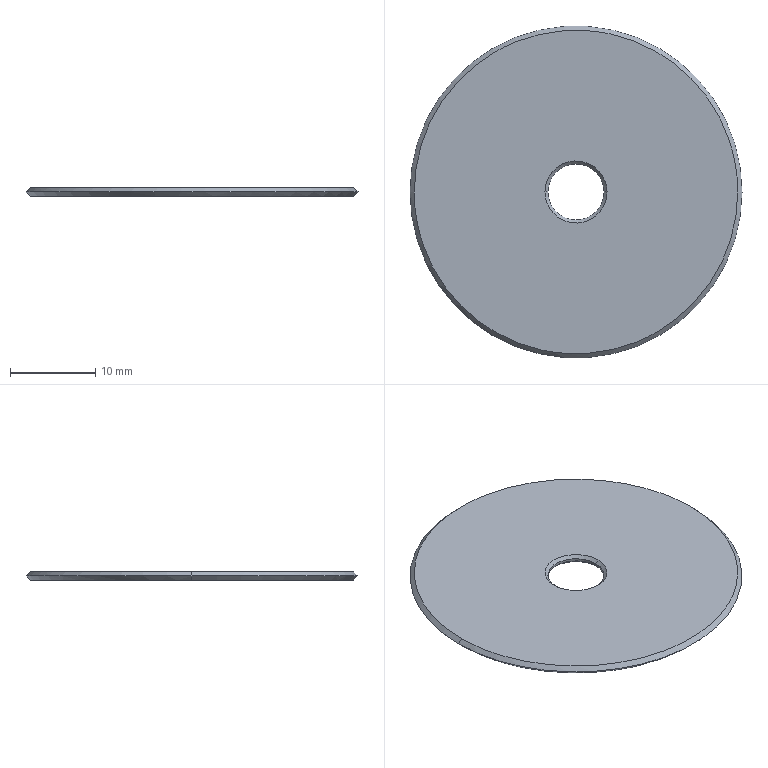Part | STEP file | Apoio de Suporte_1-A | 1 solid | 12 faces | box 39 x 39 x 1 mm | volume 1127 mm3 | cone 8 | cylinder 2 | plane 2 | commonest cylinder face diameters 6.6 x2